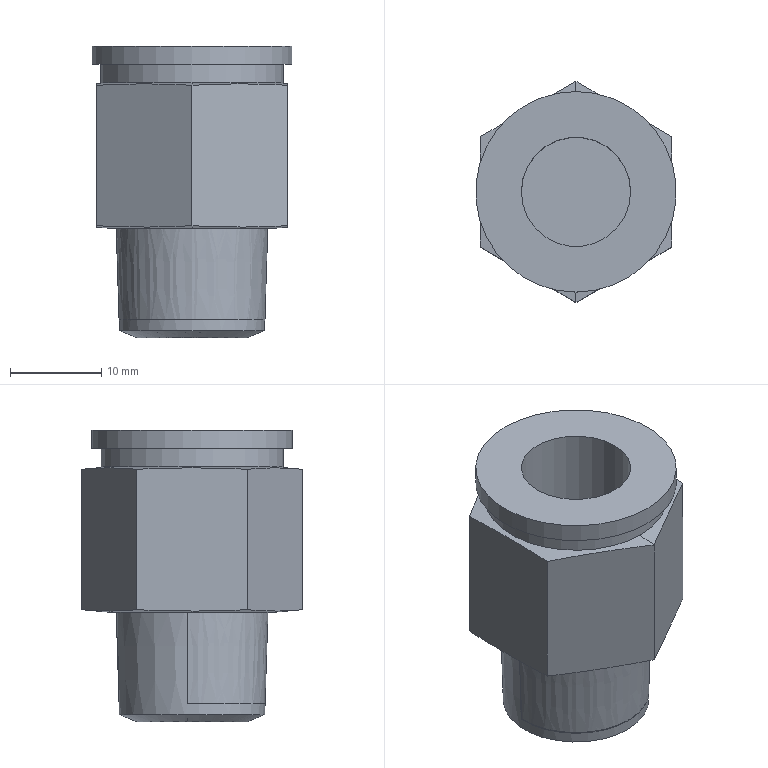Part | STEP file | EN53801200 | 2 solids | 79 faces | box 22 x 24.249 x 32.01 mm | volume 7856 mm3 | plane 38 | cone 16 | other 16 | cylinder 5 | spline 4 | commonest cylinder face diameters 12 x2 11 x1 20 x1 22 x1